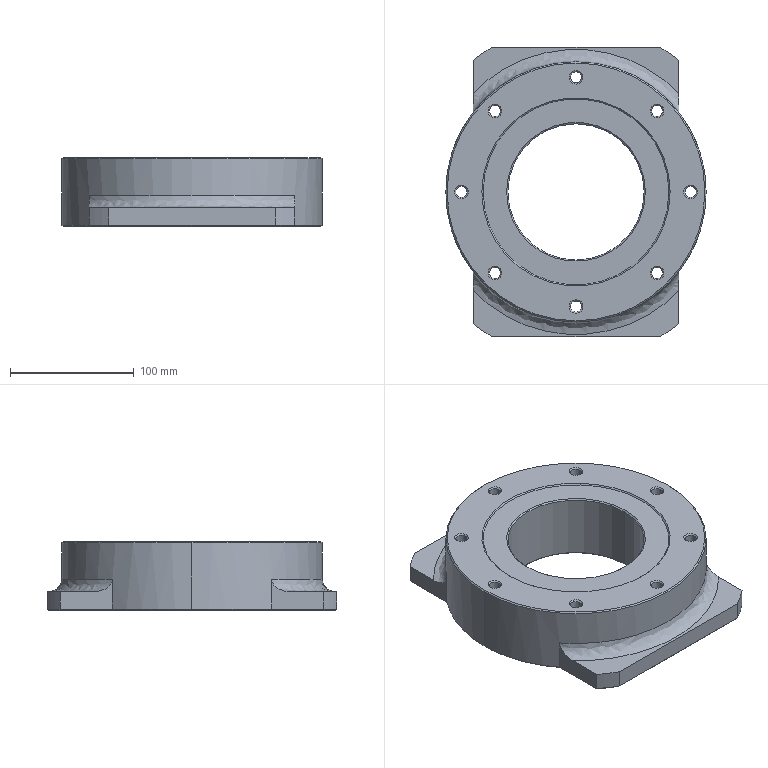Part | SolidWorks | features BaseBody 1 | 1 solid | 137 faces | box 210 x 234 x 55.5 mm | volume 1439781 mm3 | cone 57 | cylinder 48 | plane 30 | spline 2 | commonest cylinder face diameters 9 x16 14.5 x16 6.5 x8 270 x4 110 x2 210 x2